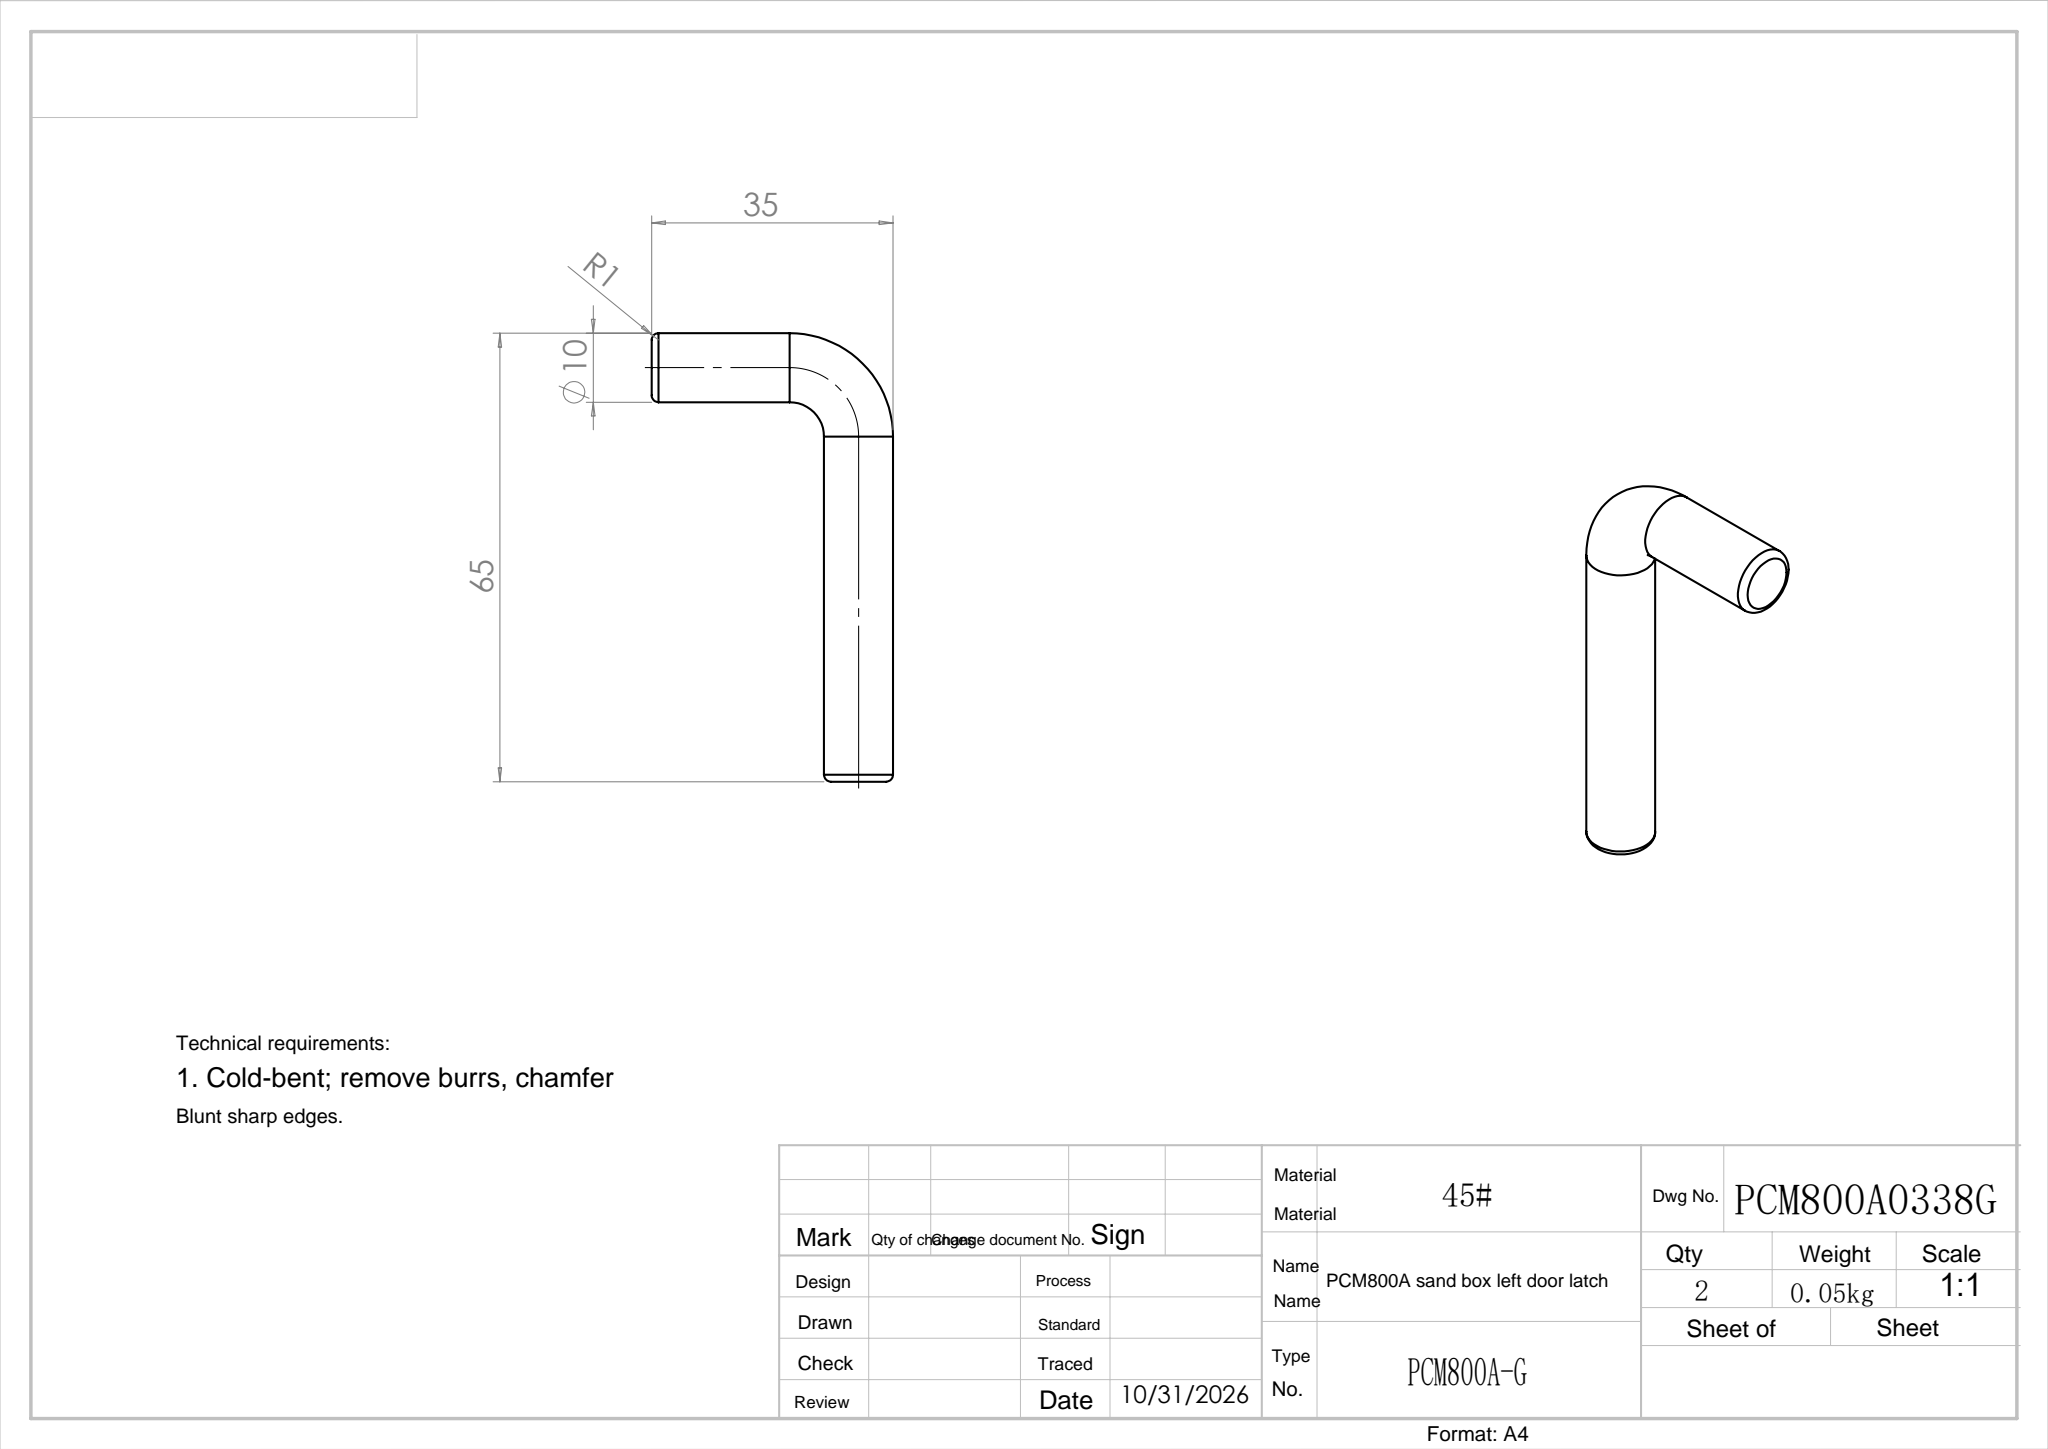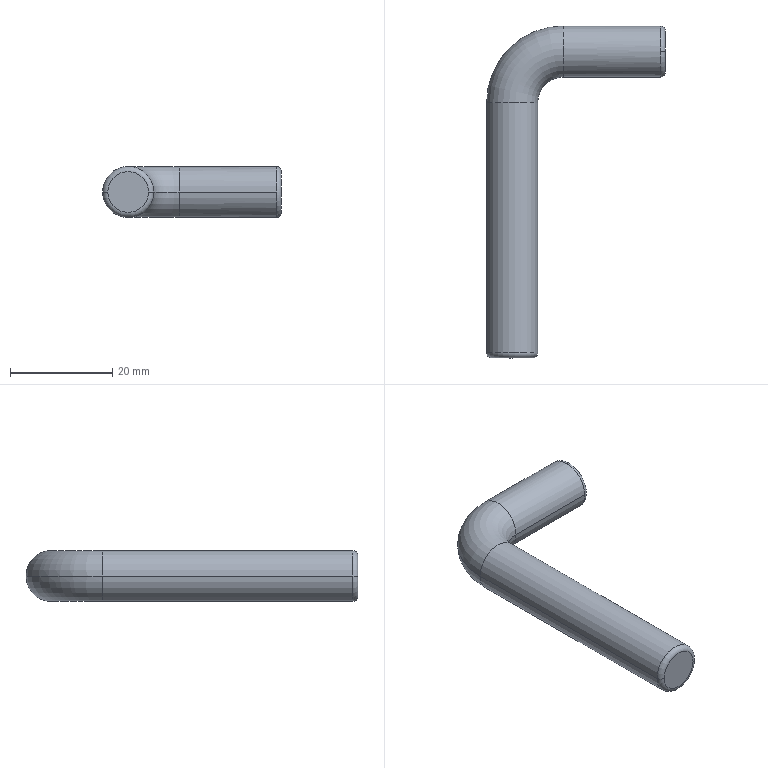Part | SolidWorks | features Fillet 1, Sweep 1 | 1 solid | 12 faces | box 35 x 65 x 10 mm | volume 6719 mm3 | torus 6 | cylinder 4 | plane 2 | commonest cylinder face diameters 10 x4
STEP:
#1=CARTESIAN_POINT('',(-20.,5.,0.));
#2=VERTEX_POINT('',#1);
#3=CARTESIAN_POINT('',(-20.,-5.,0.));
#4=VERTEX_POINT('',#3);
#5=CARTESIAN_POINT('',(-20.,0.,0.));
#6=DIRECTION('',(1.,0.,0.));
#7=DIRECTION('',(0.,0.,-1.));
#8=AXIS2_PLACEMENT_3D('',#5,#6,#7);
#9=CIRCLE('',#8,5.);
#10=EDGE_CURVE('',#2,#4,#9,.T.);
#11=ORIENTED_EDGE('',*,*,#10,.F.);
#12=CARTESIAN_POINT('',(-35.,-10.,0.));
#13=VERTEX_POINT('',#12);
#14=CARTESIAN_POINT('',(-20.,-10.,0.));
#15=DIRECTION('',(0.,0.,1.));
#16=DIRECTION('',(1.,0.,0.));
#17=AXIS2_PLACEMENT_3D('',#14,#15,#16);
#18=CIRCLE('',#17,15.);
#19=EDGE_CURVE('',#2,#13,#18,.T.);
#20=ORIENTED_EDGE('',*,*,#19,.T.);
#21=CARTESIAN_POINT('',(-25.,-10.,0.));
#22=VERTEX_POINT('',#21);
#23=CARTESIAN_POINT('',(-30.,-10.,0.));
#24=DIRECTION('',(0.,1.,0.));
#25=DIRECTION('',(0.,0.,-1.));
#26=AXIS2_PLACEMENT_3D('',#23,#24,#25);
#27=CIRCLE('',#26,5.);
#28=EDGE_CURVE('',#13,#22,#27,.T.);
#29=ORIENTED_EDGE('',*,*,#28,.T.);
#30=CARTESIAN_POINT('',(-20.,-10.,0.));
#31=DIRECTION('',(0.,0.,1.));
#32=DIRECTION('',(1.,0.,0.));
#33=AXIS2_PLACEMENT_3D('',#30,#31,#32);
#34=CIRCLE('',#33,5.);
#35=EDGE_CURVE('',#4,#22,#34,.T.);
#36=ORIENTED_EDGE('',*,*,#35,.F.);
#37=EDGE_LOOP('',(#11,#20,#29,#36));
#38=FACE_OUTER_BOUND('',#37,.T.);
#39=CARTESIAN_POINT('',(-20.,-10.,0.));
#40=DIRECTION('',(0.,0.,1.));
#41=DIRECTION('',(1.,0.,0.));
#42=AXIS2_PLACEMENT_3D('',#39,#40,#41);
#43=TOROIDAL_SURFACE('',#42,10.,5.);
#44=ADVANCED_FACE('',(#38),#43,.T.);
#45=CARTESIAN_POINT('',(-1.,0.,5.));
#46=VERTEX_POINT('',#45);
#47=CARTESIAN_POINT('',(-1.,5.,0.));
#48=VERTEX_POINT('',#47);
#49=CARTESIAN_POINT('',(-1.,0.,0.));
#50=DIRECTION('',(-1.,0.,0.));
#51=DIRECTION('',(0.,0.,-1.));
#52=AXIS2_PLACEMENT_3D('',#49,#50,#51);
#53=CIRCLE('',#52,5.);
#54=EDGE_CURVE('',#46,#48,#53,.T.);
#55=ORIENTED_EDGE('',*,*,#54,.F.);
#56=CARTESIAN_POINT('',(0.,0.,4.));
#57=VERTEX_POINT('',#56);
#58=CARTESIAN_POINT('',(-1.,0.,4.));
#59=DIRECTION('',(0.,1.,0.));
#60=DIRECTION('',(0.,0.,1.));
#61=AXIS2_PLACEMENT_3D('',#58,#59,#60);
#62=CIRCLE('',#61,1.);
#63=EDGE_CURVE('',#46,#57,#62,.T.);
#64=ORIENTED_EDGE('',*,*,#63,.T.);
#65=CARTESIAN_POINT('',(0.,0.,-4.));
#66=VERTEX_POINT('',#65);
#67=CARTESIAN_POINT('',(0.,0.,0.));
#68=DIRECTION('',(1.,0.,0.));
#69=DIRECTION('',(0.,0.,-1.));
#70=AXIS2_PLACEMENT_3D('',#67,#68,#69);
#71=CIRCLE('',#70,4.);
#72=EDGE_CURVE('',#66,#57,#71,.T.);
#73=ORIENTED_EDGE('',*,*,#72,.F.);
#74=CARTESIAN_POINT('',(-1.,0.,-5.));
#75=VERTEX_POINT('',#74);
#76=CARTESIAN_POINT('',(-1.,0.,-4.));
#77=DIRECTION('',(0.,-1.,0.));
#78=DIRECTION('',(0.,0.,-1.));
#79=AXIS2_PLACEMENT_3D('',#76,#77,#78);
#80=CIRCLE('',#79,1.);
#81=EDGE_CURVE('',#75,#66,#80,.T.);
#82=ORIENTED_EDGE('',*,*,#81,.F.);
#83=CARTESIAN_POINT('',(-1.,0.,0.));
#84=DIRECTION('',(-1.,0.,0.));
#85=DIRECTION('',(0.,0.,-1.));
#86=AXIS2_PLACEMENT_3D('',#83,#84,#85);
#87=CIRCLE('',#86,5.);
#88=EDGE_CURVE('',#48,#75,#87,.T.);
#89=ORIENTED_EDGE('',*,*,#88,.F.);
#90=EDGE_LOOP('',(#55,#64,#73,#82,#89));
#91=FACE_OUTER_BOUND('',#90,.T.);
#92=CARTESIAN_POINT('',(-1.,0.,0.));
#93=DIRECTION('',(1.,0.,0.));
#94=DIRECTION('',(0.,0.,-1.));
#95=AXIS2_PLACEMENT_3D('',#92,#93,#94);
#96=TOROIDAL_SURFACE('',#95,4.,1.);
#97=ADVANCED_FACE('',(#91),#96,.T.);
#98=CARTESIAN_POINT('',(-26.,-60.,0.));
#99=VERTEX_POINT('',#98);
#100=CARTESIAN_POINT('',(-34.,-60.,0.));
#101=VERTEX_POINT('',#100);
#102=CARTESIAN_POINT('',(-30.,-60.,0.));
#103=DIRECTION('',(0.,-1.,0.));
#104=DIRECTION('',(-1.,0.,0.));
#105=AXIS2_PLACEMENT_3D('',#102,#103,#104);
#106=CIRCLE('',#105,4.);
#107=EDGE_CURVE('',#99,#101,#106,.T.);
#108=ORIENTED_EDGE('',*,*,#107,.F.);
#109=CARTESIAN_POINT('',(-25.,-59.,0.));
#110=VERTEX_POINT('',#109);
#111=CARTESIAN_POINT('',(-26.,-59.,0.));
#112=DIRECTION('',(0.,0.,1.));
#113=DIRECTION('',(1.,0.,0.));
#114=AXIS2_PLACEMENT_3D('',#111,#112,#113);
#115=CIRCLE('',#114,1.);
#116=EDGE_CURVE('',#99,#110,#115,.T.);
#117=ORIENTED_EDGE('',*,*,#116,.T.);
#118=CARTESIAN_POINT('',(-35.,-59.,0.));
#119=VERTEX_POINT('',#118);
#120=CARTESIAN_POINT('',(-30.,-59.,0.));
#121=DIRECTION('',(0.,1.,0.));
#122=DIRECTION('',(-1.,0.,0.));
#123=AXIS2_PLACEMENT_3D('',#120,#121,#122);
#124=CIRCLE('',#123,5.);
#125=EDGE_CURVE('',#119,#110,#124,.T.);
#126=ORIENTED_EDGE('',*,*,#125,.F.);
#127=CARTESIAN_POINT('',(-34.,-59.,0.));
#128=DIRECTION('',(0.,0.,-1.));
#129=DIRECTION('',(-1.,0.,0.));
#130=AXIS2_PLACEMENT_3D('',#127,#128,#129);
#131=CIRCLE('',#130,1.);
#132=EDGE_CURVE('',#101,#119,#131,.T.);
#133=ORIENTED_EDGE('',*,*,#132,.F.);
#134=EDGE_LOOP('',(#108,#117,#126,#133));
#135=FACE_OUTER_BOUND('',#134,.T.);
#136=CARTESIAN_POINT('',(-30.,-59.,0.));
#137=DIRECTION('',(0.,1.,0.));
#138=DIRECTION('',(-1.,0.,0.));
#139=AXIS2_PLACEMENT_3D('',#136,#137,#138);
#140=TOROIDAL_SURFACE('',#139,4.,1.);
#141=ADVANCED_FACE('',(#135),#140,.T.);
#142=ORIENTED_EDGE('',*,*,#10,.T.);
#143=CARTESIAN_POINT('',(-1.,-5.,0.));
#144=VERTEX_POINT('',#143);
#145=CARTESIAN_POINT('',(-20.,-5.,0.));
#146=DIRECTION('',(1.,0.,0.));
#147=VECTOR('',#146,1000.);
#148=LINE('',#145,#147);
#149=EDGE_CURVE('',#4,#144,#148,.T.);
#150=ORIENTED_EDGE('',*,*,#149,.T.);
#151=CARTESIAN_POINT('',(-1.,0.,0.));
#152=DIRECTION('',(-1.,0.,0.));
#153=DIRECTION('',(0.,0.,-1.));
#154=AXIS2_PLACEMENT_3D('',#151,#152,#153);
#155=CIRCLE('',#154,5.);
#156=EDGE_CURVE('',#144,#46,#155,.T.);
#157=ORIENTED_EDGE('',*,*,#156,.T.);
#158=ORIENTED_EDGE('',*,*,#54,.T.);
#159=CARTESIAN_POINT('',(-20.,5.,0.));
#160=DIRECTION('',(1.,0.,0.));
#161=VECTOR('',#160,1000.);
#162=LINE('',#159,#161);
#163=EDGE_CURVE('',#2,#48,#162,.T.);
#164=ORIENTED_EDGE('',*,*,#163,.F.);
#165=EDGE_LOOP('',(#142,#150,#157,#158,#164));
#166=FACE_OUTER_BOUND('',#165,.T.);
#167=CARTESIAN_POINT('',(-20.,0.,0.));
#168=DIRECTION('',(1.,0.,0.));
#169=DIRECTION('',(0.,1.,0.));
#170=AXIS2_PLACEMENT_3D('',#167,#168,#169);
#171=CYLINDRICAL_SURFACE('',#170,5.);
#172=ADVANCED_FACE('',(#166),#171,.T.);
#173=ORIENTED_EDGE('',*,*,#28,.F.);
#174=CARTESIAN_POINT('',(-35.,-10.,0.));
#175=DIRECTION('',(0.,-1.,0.));
#176=VECTOR('',#175,1000.);
#177=LINE('',#174,#176);
#178=EDGE_CURVE('',#13,#119,#177,.T.);
#179=ORIENTED_EDGE('',*,*,#178,.T.);
#180=ORIENTED_EDGE('',*,*,#125,.T.);
#181=CARTESIAN_POINT('',(-25.,-10.,0.));
#182=DIRECTION('',(0.,-1.,0.));
#183=VECTOR('',#182,1000.);
#184=LINE('',#181,#183);
#185=EDGE_CURVE('',#22,#110,#184,.T.);
#186=ORIENTED_EDGE('',*,*,#185,.F.);
#187=EDGE_LOOP('',(#173,#179,#180,#186));
#188=FACE_OUTER_BOUND('',#187,.T.);
#189=CARTESIAN_POINT('',(-30.,-10.,0.));
#190=DIRECTION('',(0.,-1.,0.));
#191=DIRECTION('',(1.,0.,0.));
#192=AXIS2_PLACEMENT_3D('',#189,#190,#191);
#193=CYLINDRICAL_SURFACE('',#192,5.);
#194=ADVANCED_FACE('',(#188),#193,.T.);
#195=ORIENTED_EDGE('',*,*,#178,.F.);
#196=CARTESIAN_POINT('',(-30.,-10.,0.));
#197=DIRECTION('',(0.,1.,0.));
#198=DIRECTION('',(0.,0.,-1.));
#199=AXIS2_PLACEMENT_3D('',#196,#197,#198);
#200=CIRCLE('',#199,5.);
#201=EDGE_CURVE('',#22,#13,#200,.T.);
#202=ORIENTED_EDGE('',*,*,#201,.F.);
#203=ORIENTED_EDGE('',*,*,#185,.T.);
#204=CARTESIAN_POINT('',(-30.,-59.,0.));
#205=DIRECTION('',(0.,1.,0.));
#206=DIRECTION('',(-1.,0.,0.));
#207=AXIS2_PLACEMENT_3D('',#204,#205,#206);
#208=CIRCLE('',#207,5.);
#209=EDGE_CURVE('',#110,#119,#208,.T.);
#210=ORIENTED_EDGE('',*,*,#209,.T.);
#211=EDGE_LOOP('',(#195,#202,#203,#210));
#212=FACE_OUTER_BOUND('',#211,.T.);
#213=CARTESIAN_POINT('',(-30.,-10.,0.));
#214=DIRECTION('',(0.,-1.,0.));
#215=DIRECTION('',(1.,0.,0.));
#216=AXIS2_PLACEMENT_3D('',#213,#214,#215);
#217=CYLINDRICAL_SURFACE('',#216,5.);
#218=ADVANCED_FACE('',(#212),#217,.T.);
#219=ORIENTED_EDGE('',*,*,#19,.F.);
#220=CARTESIAN_POINT('',(-20.,0.,0.));
#221=DIRECTION('',(1.,0.,0.));
#222=DIRECTION('',(0.,0.,-1.));
#223=AXIS2_PLACEMENT_3D('',#220,#221,#222);
#224=CIRCLE('',#223,5.);
#225=EDGE_CURVE('',#4,#2,#224,.T.);
#226=ORIENTED_EDGE('',*,*,#225,.F.);
#227=ORIENTED_EDGE('',*,*,#35,.T.);
#228=ORIENTED_EDGE('',*,*,#201,.T.);
#229=EDGE_LOOP('',(#219,#226,#227,#228));
#230=FACE_OUTER_BOUND('',#229,.T.);
#231=CARTESIAN_POINT('',(-20.,-10.,0.));
#232=DIRECTION('',(0.,0.,1.));
#233=DIRECTION('',(1.,0.,0.));
#234=AXIS2_PLACEMENT_3D('',#231,#232,#233);
#235=TOROIDAL_SURFACE('',#234,10.,5.);
#236=ADVANCED_FACE('',(#230),#235,.T.);
#237=ORIENTED_EDGE('',*,*,#149,.F.);
#238=ORIENTED_EDGE('',*,*,#225,.T.);
#239=ORIENTED_EDGE('',*,*,#163,.T.);
#240=ORIENTED_EDGE('',*,*,#88,.T.);
#241=CARTESIAN_POINT('',(-1.,0.,0.));
#242=DIRECTION('',(-1.,0.,0.));
#243=DIRECTION('',(0.,0.,-1.));
#244=AXIS2_PLACEMENT_3D('',#241,#242,#243);
#245=CIRCLE('',#244,5.);
#246=EDGE_CURVE('',#75,#144,#245,.T.);
#247=ORIENTED_EDGE('',*,*,#246,.T.);
#248=EDGE_LOOP('',(#237,#238,#239,#240,#247));
#249=FACE_OUTER_BOUND('',#248,.T.);
#250=CARTESIAN_POINT('',(-20.,0.,0.));
#251=DIRECTION('',(1.,0.,0.));
#252=DIRECTION('',(0.,1.,0.));
#253=AXIS2_PLACEMENT_3D('',#250,#251,#252);
#254=CYLINDRICAL_SURFACE('',#253,5.);
#255=ADVANCED_FACE('',(#249),#254,.T.);
#256=CARTESIAN_POINT('',(-30.,-60.,0.));
#257=DIRECTION('',(0.,-1.,0.));
#258=DIRECTION('',(-1.,0.,0.));
#259=AXIS2_PLACEMENT_3D('',#256,#257,#258);
#260=CIRCLE('',#259,4.);
#261=EDGE_CURVE('',#101,#99,#260,.T.);
#262=ORIENTED_EDGE('',*,*,#261,.T.);
#263=ORIENTED_EDGE('',*,*,#107,.T.);
#264=EDGE_LOOP('',(#262,#263));
#265=FACE_OUTER_BOUND('',#264,.T.);
#266=CARTESIAN_POINT('',(-30.,-60.,0.));
#267=DIRECTION('',(0.,1.,0.));
#268=DIRECTION('',(0.,0.,-1.));
#269=AXIS2_PLACEMENT_3D('',#266,#267,#268);
#270=PLANE('',#269);
#271=ADVANCED_FACE('',(#265),#270,.F.);
#272=ORIENTED_EDGE('',*,*,#72,.T.);
#273=CARTESIAN_POINT('',(0.,0.,0.));
#274=DIRECTION('',(1.,0.,0.));
#275=DIRECTION('',(0.,0.,-1.));
#276=AXIS2_PLACEMENT_3D('',#273,#274,#275);
#277=CIRCLE('',#276,4.);
#278=EDGE_CURVE('',#57,#66,#277,.T.);
#279=ORIENTED_EDGE('',*,*,#278,.T.);
#280=EDGE_LOOP('',(#272,#279));
#281=FACE_OUTER_BOUND('',#280,.T.);
#282=CARTESIAN_POINT('',(0.,0.,0.));
#283=DIRECTION('',(1.,0.,0.));
#284=DIRECTION('',(0.,0.,-1.));
#285=AXIS2_PLACEMENT_3D('',#282,#283,#284);
#286=PLANE('',#285);
#287=ADVANCED_FACE('',(#281),#286,.T.);
#288=ORIENTED_EDGE('',*,*,#116,.F.);
#289=ORIENTED_EDGE('',*,*,#261,.F.);
#290=ORIENTED_EDGE('',*,*,#132,.T.);
#291=ORIENTED_EDGE('',*,*,#209,.F.);
#292=EDGE_LOOP('',(#288,#289,#290,#291));
#293=FACE_OUTER_BOUND('',#292,.T.);
#294=CARTESIAN_POINT('',(-30.,-59.,0.));
#295=DIRECTION('',(0.,1.,0.));
#296=DIRECTION('',(-1.,0.,0.));
#297=AXIS2_PLACEMENT_3D('',#294,#295,#296);
#298=TOROIDAL_SURFACE('',#297,4.,1.);
#299=ADVANCED_FACE('',(#293),#298,.T.);
#300=ORIENTED_EDGE('',*,*,#63,.F.);
#301=ORIENTED_EDGE('',*,*,#156,.F.);
#302=ORIENTED_EDGE('',*,*,#246,.F.);
#303=ORIENTED_EDGE('',*,*,#81,.T.);
#304=ORIENTED_EDGE('',*,*,#278,.F.);
#305=EDGE_LOOP('',(#300,#301,#302,#303,#304));
#306=FACE_OUTER_BOUND('',#305,.T.);
#307=CARTESIAN_POINT('',(-1.,0.,0.));
#308=DIRECTION('',(1.,0.,0.));
#309=DIRECTION('',(0.,0.,-1.));
#310=AXIS2_PLACEMENT_3D('',#307,#308,#309);
#311=TOROIDAL_SURFACE('',#310,4.,1.);
#312=ADVANCED_FACE('',(#306),#311,.T.);
#313=CLOSED_SHELL('',(#44,#97,#141,#172,#194,#218,#236,#255,#271,#287,#299,#312));
#314=MANIFOLD_SOLID_BREP('',#313);
#315=CARTESIAN_POINT('',(0.,0.,0.));
#316=DIRECTION('',(0.,0.,1.));
#317=DIRECTION('',(1.,0.,0.));
#318=AXIS2_PLACEMENT_3D('',#315,#316,#317);
#319=(LENGTH_UNIT()NAMED_UNIT(*)SI_UNIT(.MILLI.,.METRE.));
#320=UNCERTAINTY_MEASURE_WITH_UNIT(LENGTH_MEASURE(0.00001),#319,'','');
#321=(NAMED_UNIT(*)PLANE_ANGLE_UNIT()SI_UNIT($,.RADIAN.));
#322=(NAMED_UNIT(*)SI_UNIT($,.STERADIAN.)SOLID_ANGLE_UNIT());
#323=(GEOMETRIC_REPRESENTATION_CONTEXT(3)GLOBAL_UNCERTAINTY_ASSIGNED_CONTEXT((#320))GLOBAL_UNIT_ASSIGNED_CONTEXT((#319,#321,#322))REPRESENTATION_CONTEXT('',''));
#324=ADVANCED_BREP_SHAPE_REPRESENTATION('',(#314,#318),#323);